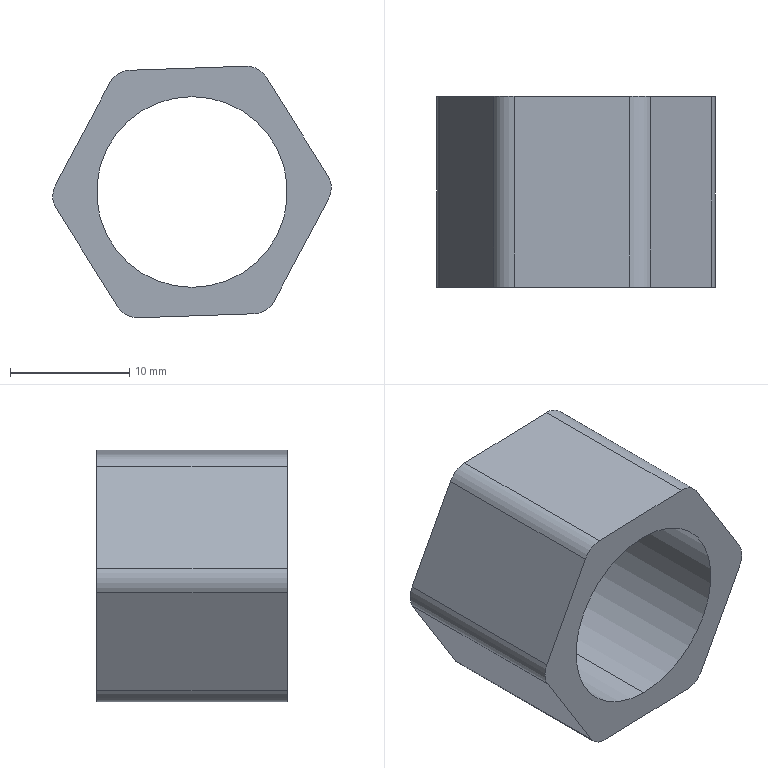Part | SolidWorks | features Fillet 2, Extrusion 1 | 1 solid | 17 faces | box 23.37 x 16 x 21.11 mm | volume 2748 mm3 | cylinder 9 | plane 8 | commonest cylinder face diameters 4 x7 16 x2
STEP:
#1=CARTESIAN_POINT('',(-4.552,16.,-10.555));
#2=VERTEX_POINT('',#1);
#3=CARTESIAN_POINT('',(-6.249,16.,-9.614));
#4=VERTEX_POINT('',#3);
#5=CARTESIAN_POINT('',(-4.552,16.,-8.555));
#6=DIRECTION('',(0.,1.,0.));
#7=DIRECTION('',(0.,0.,1.));
#8=AXIS2_PLACEMENT_3D('',#5,#6,#7);
#9=CIRCLE('',#8,2.);
#10=EDGE_CURVE('',#2,#4,#9,.T.);
#11=ORIENTED_EDGE('',*,*,#10,.F.);
#12=CARTESIAN_POINT('',(-4.552,0.,-10.555));
#13=VERTEX_POINT('',#12);
#14=CARTESIAN_POINT('',(-4.552,16.,-10.555));
#15=DIRECTION('',(0.,-1.,0.));
#16=VECTOR('',#15,1000.);
#17=LINE('',#14,#16);
#18=EDGE_CURVE('',#2,#13,#17,.T.);
#19=ORIENTED_EDGE('',*,*,#18,.T.);
#20=CARTESIAN_POINT('',(-6.249,0.,-9.614));
#21=VERTEX_POINT('',#20);
#22=CARTESIAN_POINT('',(-4.552,0.,-8.555));
#23=DIRECTION('',(0.,-1.,0.));
#24=DIRECTION('',(0.,0.,1.));
#25=AXIS2_PLACEMENT_3D('',#22,#23,#24);
#26=CIRCLE('',#25,2.);
#27=EDGE_CURVE('',#21,#13,#26,.T.);
#28=ORIENTED_EDGE('',*,*,#27,.F.);
#29=CARTESIAN_POINT('',(-6.249,16.,-9.614));
#30=DIRECTION('',(0.,-1.,0.));
#31=VECTOR('',#30,1000.);
#32=LINE('',#29,#31);
#33=EDGE_CURVE('',#4,#21,#32,.T.);
#34=ORIENTED_EDGE('',*,*,#33,.F.);
#35=EDGE_LOOP('',(#11,#19,#28,#34));
#36=FACE_OUTER_BOUND('',#35,.T.);
#37=CARTESIAN_POINT('',(-4.552,16.,-8.555));
#38=DIRECTION('',(0.,-1.,0.));
#39=DIRECTION('',(0.,0.,-1.));
#40=AXIS2_PLACEMENT_3D('',#37,#38,#39);
#41=CYLINDRICAL_SURFACE('',#40,2.);
#42=ADVANCED_FACE('',(#36),#41,.T.);
#43=CARTESIAN_POINT('',(0.,16.,-8.));
#44=VERTEX_POINT('',#43);
#45=CARTESIAN_POINT('',(0.,16.,8.));
#46=VERTEX_POINT('',#45);
#47=CARTESIAN_POINT('',(0.,16.,0.));
#48=DIRECTION('',(0.,1.,0.));
#49=DIRECTION('',(0.,0.,1.));
#50=AXIS2_PLACEMENT_3D('',#47,#48,#49);
#51=CIRCLE('',#50,8.);
#52=EDGE_CURVE('',#44,#46,#51,.T.);
#53=ORIENTED_EDGE('',*,*,#52,.T.);
#54=CARTESIAN_POINT('',(0.,0.,8.));
#55=VERTEX_POINT('',#54);
#56=CARTESIAN_POINT('',(0.,16.,8.));
#57=DIRECTION('',(0.,-1.,0.));
#58=VECTOR('',#57,1000.);
#59=LINE('',#56,#58);
#60=EDGE_CURVE('',#46,#55,#59,.T.);
#61=ORIENTED_EDGE('',*,*,#60,.T.);
#62=CARTESIAN_POINT('',(0.,0.,-8.));
#63=VERTEX_POINT('',#62);
#64=CARTESIAN_POINT('',(0.,0.,0.));
#65=DIRECTION('',(0.,1.,0.));
#66=DIRECTION('',(0.,0.,1.));
#67=AXIS2_PLACEMENT_3D('',#64,#65,#66);
#68=CIRCLE('',#67,8.);
#69=EDGE_CURVE('',#63,#55,#68,.T.);
#70=ORIENTED_EDGE('',*,*,#69,.F.);
#71=CARTESIAN_POINT('',(0.,16.,-8.));
#72=DIRECTION('',(0.,-1.,0.));
#73=VECTOR('',#72,1000.);
#74=LINE('',#71,#73);
#75=EDGE_CURVE('',#44,#63,#74,.T.);
#76=ORIENTED_EDGE('',*,*,#75,.F.);
#77=EDGE_LOOP('',(#53,#61,#70,#76));
#78=FACE_OUTER_BOUND('',#77,.T.);
#79=CARTESIAN_POINT('',(0.,16.,0.));
#80=DIRECTION('',(0.,-1.,0.));
#81=DIRECTION('',(0.,0.,-1.));
#82=AXIS2_PLACEMENT_3D('',#79,#80,#81);
#83=CYLINDRICAL_SURFACE('',#82,8.);
#84=ADVANCED_FACE('',(#78),#83,.F.);
#85=CARTESIAN_POINT('',(5.202,16.,-10.219));
#86=VERTEX_POINT('',#85);
#87=CARTESIAN_POINT('',(-4.483,16.,-10.554));
#88=VERTEX_POINT('',#87);
#89=CARTESIAN_POINT('',(6.356,16.,-10.179));
#90=DIRECTION('',(-0.9994,0.,-0.03459));
#91=VECTOR('',#90,1000.);
#92=LINE('',#89,#91);
#93=EDGE_CURVE('',#86,#88,#92,.T.);
#94=ORIENTED_EDGE('',*,*,#93,.T.);
#95=CARTESIAN_POINT('',(-4.552,16.,-8.555));
#96=DIRECTION('',(0.,1.,0.));
#97=DIRECTION('',(0.,0.,1.));
#98=AXIS2_PLACEMENT_3D('',#95,#96,#97);
#99=CIRCLE('',#98,2.);
#100=EDGE_CURVE('',#88,#2,#99,.T.);
#101=ORIENTED_EDGE('',*,*,#100,.T.);
#102=ORIENTED_EDGE('',*,*,#10,.T.);
#103=CARTESIAN_POINT('',(-11.381,16.,-1.394));
#104=VERTEX_POINT('',#103);
#105=CARTESIAN_POINT('',(-5.637,16.,-10.594));
#106=DIRECTION('',(-0.5297,0.,0.8482));
#107=VECTOR('',#106,1000.);
#108=LINE('',#105,#107);
#109=EDGE_CURVE('',#4,#104,#108,.T.);
#110=ORIENTED_EDGE('',*,*,#109,.T.);
#111=CARTESIAN_POINT('',(-11.45,16.,0.6043));
#112=VERTEX_POINT('',#111);
#113=CARTESIAN_POINT('',(-9.685,16.,-0.3352));
#114=DIRECTION('',(0.,1.,0.));
#115=DIRECTION('',(0.,0.,1.));
#116=AXIS2_PLACEMENT_3D('',#113,#114,#115);
#117=CIRCLE('',#116,2.);
#118=EDGE_CURVE('',#104,#112,#117,.T.);
#119=ORIENTED_EDGE('',*,*,#118,.T.);
#120=CARTESIAN_POINT('',(-6.898,16.,9.159));
#121=VERTEX_POINT('',#120);
#122=CARTESIAN_POINT('',(-11.993,16.,-0.415));
#123=DIRECTION('',(0.4697,0.,0.8828));
#124=VECTOR('',#123,1000.);
#125=LINE('',#122,#124);
#126=EDGE_CURVE('',#112,#121,#125,.T.);
#127=ORIENTED_EDGE('',*,*,#126,.T.);
#128=CARTESIAN_POINT('',(-5.202,16.,10.219));
#129=VERTEX_POINT('',#128);
#130=CARTESIAN_POINT('',(-5.133,16.,8.22));
#131=DIRECTION('',(0.,1.,0.));
#132=DIRECTION('',(0.,0.,1.));
#133=AXIS2_PLACEMENT_3D('',#130,#131,#132);
#134=CIRCLE('',#133,2.);
#135=EDGE_CURVE('',#121,#129,#134,.T.);
#136=ORIENTED_EDGE('',*,*,#135,.T.);
#137=CARTESIAN_POINT('',(4.483,16.,10.554));
#138=VERTEX_POINT('',#137);
#139=CARTESIAN_POINT('',(-6.356,16.,10.179));
#140=DIRECTION('',(0.9994,0.,0.03459));
#141=VECTOR('',#140,1000.);
#142=LINE('',#139,#141);
#143=EDGE_CURVE('',#129,#138,#142,.T.);
#144=ORIENTED_EDGE('',*,*,#143,.T.);
#145=CARTESIAN_POINT('',(6.249,16.,9.614));
#146=VERTEX_POINT('',#145);
#147=CARTESIAN_POINT('',(4.552,16.,8.555));
#148=DIRECTION('',(0.,1.,0.));
#149=DIRECTION('',(0.,0.,1.));
#150=AXIS2_PLACEMENT_3D('',#147,#148,#149);
#151=CIRCLE('',#150,2.);
#152=EDGE_CURVE('',#138,#146,#151,.T.);
#153=ORIENTED_EDGE('',*,*,#152,.T.);
#154=CARTESIAN_POINT('',(11.381,16.,1.394));
#155=VERTEX_POINT('',#154);
#156=CARTESIAN_POINT('',(5.637,16.,10.594));
#157=DIRECTION('',(0.5297,0.,-0.8482));
#158=VECTOR('',#157,1000.);
#159=LINE('',#156,#158);
#160=EDGE_CURVE('',#146,#155,#159,.T.);
#161=ORIENTED_EDGE('',*,*,#160,.T.);
#162=CARTESIAN_POINT('',(11.45,16.,-0.6043));
#163=VERTEX_POINT('',#162);
#164=CARTESIAN_POINT('',(9.685,16.,0.3352));
#165=DIRECTION('',(0.,1.,0.));
#166=DIRECTION('',(0.,0.,1.));
#167=AXIS2_PLACEMENT_3D('',#164,#165,#166);
#168=CIRCLE('',#167,2.);
#169=EDGE_CURVE('',#155,#163,#168,.T.);
#170=ORIENTED_EDGE('',*,*,#169,.T.);
#171=CARTESIAN_POINT('',(6.898,16.,-9.159));
#172=VERTEX_POINT('',#171);
#173=CARTESIAN_POINT('',(11.993,16.,0.415));
#174=DIRECTION('',(-0.4697,0.,-0.8828));
#175=VECTOR('',#174,1000.);
#176=LINE('',#173,#175);
#177=EDGE_CURVE('',#163,#172,#176,.T.);
#178=ORIENTED_EDGE('',*,*,#177,.T.);
#179=CARTESIAN_POINT('',(5.133,16.,-8.22));
#180=DIRECTION('',(0.,1.,0.));
#181=DIRECTION('',(0.,0.,1.));
#182=AXIS2_PLACEMENT_3D('',#179,#180,#181);
#183=CIRCLE('',#182,2.);
#184=EDGE_CURVE('',#172,#86,#183,.T.);
#185=ORIENTED_EDGE('',*,*,#184,.T.);
#186=EDGE_LOOP('',(#94,#101,#102,#110,#119,#127,#136,#144,#153,#161,#170,#178,#185));
#187=FACE_OUTER_BOUND('',#186,.T.);
#188=ORIENTED_EDGE('',*,*,#52,.F.);
#189=CARTESIAN_POINT('',(0.,16.,0.));
#190=DIRECTION('',(0.,1.,0.));
#191=DIRECTION('',(0.,0.,1.));
#192=AXIS2_PLACEMENT_3D('',#189,#190,#191);
#193=CIRCLE('',#192,8.);
#194=EDGE_CURVE('',#46,#44,#193,.T.);
#195=ORIENTED_EDGE('',*,*,#194,.F.);
#196=EDGE_LOOP('',(#188,#195));
#197=FACE_BOUND('',#196,.T.);
#198=CARTESIAN_POINT('',(0.,16.,0.));
#199=DIRECTION('',(0.,1.,0.));
#200=DIRECTION('',(0.,0.,1.));
#201=AXIS2_PLACEMENT_3D('',#198,#199,#200);
#202=PLANE('',#201);
#203=ADVANCED_FACE('',(#187,#197),#202,.T.);
#204=CARTESIAN_POINT('',(-11.381,0.,-1.394));
#205=VERTEX_POINT('',#204);
#206=CARTESIAN_POINT('',(-5.637,0.,-10.594));
#207=DIRECTION('',(-0.5297,0.,0.8482));
#208=VECTOR('',#207,1000.);
#209=LINE('',#206,#208);
#210=EDGE_CURVE('',#21,#205,#209,.T.);
#211=ORIENTED_EDGE('',*,*,#210,.F.);
#212=ORIENTED_EDGE('',*,*,#27,.T.);
#213=CARTESIAN_POINT('',(-4.483,0.,-10.554));
#214=VERTEX_POINT('',#213);
#215=CARTESIAN_POINT('',(-4.552,0.,-8.555));
#216=DIRECTION('',(0.,-1.,0.));
#217=DIRECTION('',(0.,0.,1.));
#218=AXIS2_PLACEMENT_3D('',#215,#216,#217);
#219=CIRCLE('',#218,2.);
#220=EDGE_CURVE('',#13,#214,#219,.T.);
#221=ORIENTED_EDGE('',*,*,#220,.T.);
#222=CARTESIAN_POINT('',(5.202,0.,-10.219));
#223=VERTEX_POINT('',#222);
#224=CARTESIAN_POINT('',(6.356,0.,-10.179));
#225=DIRECTION('',(-0.9994,0.,-0.03459));
#226=VECTOR('',#225,1000.);
#227=LINE('',#224,#226);
#228=EDGE_CURVE('',#223,#214,#227,.T.);
#229=ORIENTED_EDGE('',*,*,#228,.F.);
#230=CARTESIAN_POINT('',(6.898,0.,-9.159));
#231=VERTEX_POINT('',#230);
#232=CARTESIAN_POINT('',(5.133,0.,-8.22));
#233=DIRECTION('',(0.,-1.,0.));
#234=DIRECTION('',(0.,0.,1.));
#235=AXIS2_PLACEMENT_3D('',#232,#233,#234);
#236=CIRCLE('',#235,2.);
#237=EDGE_CURVE('',#223,#231,#236,.T.);
#238=ORIENTED_EDGE('',*,*,#237,.T.);
#239=CARTESIAN_POINT('',(11.45,0.,-0.6043));
#240=VERTEX_POINT('',#239);
#241=CARTESIAN_POINT('',(11.993,0.,0.415));
#242=DIRECTION('',(-0.4697,0.,-0.8828));
#243=VECTOR('',#242,1000.);
#244=LINE('',#241,#243);
#245=EDGE_CURVE('',#240,#231,#244,.T.);
#246=ORIENTED_EDGE('',*,*,#245,.F.);
#247=CARTESIAN_POINT('',(11.381,0.,1.394));
#248=VERTEX_POINT('',#247);
#249=CARTESIAN_POINT('',(9.685,0.,0.3352));
#250=DIRECTION('',(0.,-1.,0.));
#251=DIRECTION('',(0.,0.,1.));
#252=AXIS2_PLACEMENT_3D('',#249,#250,#251);
#253=CIRCLE('',#252,2.);
#254=EDGE_CURVE('',#240,#248,#253,.T.);
#255=ORIENTED_EDGE('',*,*,#254,.T.);
#256=CARTESIAN_POINT('',(6.249,0.,9.614));
#257=VERTEX_POINT('',#256);
#258=CARTESIAN_POINT('',(5.637,0.,10.594));
#259=DIRECTION('',(0.5297,0.,-0.8482));
#260=VECTOR('',#259,1000.);
#261=LINE('',#258,#260);
#262=EDGE_CURVE('',#257,#248,#261,.T.);
#263=ORIENTED_EDGE('',*,*,#262,.F.);
#264=CARTESIAN_POINT('',(4.483,0.,10.554));
#265=VERTEX_POINT('',#264);
#266=CARTESIAN_POINT('',(4.552,0.,8.555));
#267=DIRECTION('',(0.,-1.,0.));
#268=DIRECTION('',(0.,0.,1.));
#269=AXIS2_PLACEMENT_3D('',#266,#267,#268);
#270=CIRCLE('',#269,2.);
#271=EDGE_CURVE('',#257,#265,#270,.T.);
#272=ORIENTED_EDGE('',*,*,#271,.T.);
#273=CARTESIAN_POINT('',(-5.202,0.,10.219));
#274=VERTEX_POINT('',#273);
#275=CARTESIAN_POINT('',(-6.356,0.,10.179));
#276=DIRECTION('',(0.9994,0.,0.03459));
#277=VECTOR('',#276,1000.);
#278=LINE('',#275,#277);
#279=EDGE_CURVE('',#274,#265,#278,.T.);
#280=ORIENTED_EDGE('',*,*,#279,.F.);
#281=CARTESIAN_POINT('',(-6.898,0.,9.159));
#282=VERTEX_POINT('',#281);
#283=CARTESIAN_POINT('',(-5.133,0.,8.22));
#284=DIRECTION('',(0.,-1.,0.));
#285=DIRECTION('',(0.,0.,1.));
#286=AXIS2_PLACEMENT_3D('',#283,#284,#285);
#287=CIRCLE('',#286,2.);
#288=EDGE_CURVE('',#274,#282,#287,.T.);
#289=ORIENTED_EDGE('',*,*,#288,.T.);
#290=CARTESIAN_POINT('',(-11.45,0.,0.6043));
#291=VERTEX_POINT('',#290);
#292=CARTESIAN_POINT('',(-11.993,0.,-0.415));
#293=DIRECTION('',(0.4697,0.,0.8828));
#294=VECTOR('',#293,1000.);
#295=LINE('',#292,#294);
#296=EDGE_CURVE('',#291,#282,#295,.T.);
#297=ORIENTED_EDGE('',*,*,#296,.F.);
#298=CARTESIAN_POINT('',(-9.685,0.,-0.3352));
#299=DIRECTION('',(0.,-1.,0.));
#300=DIRECTION('',(0.,0.,1.));
#301=AXIS2_PLACEMENT_3D('',#298,#299,#300);
#302=CIRCLE('',#301,2.);
#303=EDGE_CURVE('',#291,#205,#302,.T.);
#304=ORIENTED_EDGE('',*,*,#303,.T.);
#305=EDGE_LOOP('',(#211,#212,#221,#229,#238,#246,#255,#263,#272,#280,#289,#297,#304));
#306=FACE_OUTER_BOUND('',#305,.T.);
#307=ORIENTED_EDGE('',*,*,#69,.T.);
#308=CARTESIAN_POINT('',(0.,0.,0.));
#309=DIRECTION('',(0.,1.,0.));
#310=DIRECTION('',(0.,0.,1.));
#311=AXIS2_PLACEMENT_3D('',#308,#309,#310);
#312=CIRCLE('',#311,8.);
#313=EDGE_CURVE('',#55,#63,#312,.T.);
#314=ORIENTED_EDGE('',*,*,#313,.T.);
#315=EDGE_LOOP('',(#307,#314));
#316=FACE_BOUND('',#315,.T.);
#317=CARTESIAN_POINT('',(0.,0.,0.));
#318=DIRECTION('',(0.,1.,0.));
#319=DIRECTION('',(0.,0.,1.));
#320=AXIS2_PLACEMENT_3D('',#317,#318,#319);
#321=PLANE('',#320);
#322=ADVANCED_FACE('',(#306,#316),#321,.F.);
#323=ORIENTED_EDGE('',*,*,#143,.F.);
#324=CARTESIAN_POINT('',(-5.202,16.,10.219));
#325=DIRECTION('',(0.,-1.,0.));
#326=VECTOR('',#325,1000.);
#327=LINE('',#324,#326);
#328=EDGE_CURVE('',#129,#274,#327,.T.);
#329=ORIENTED_EDGE('',*,*,#328,.T.);
#330=ORIENTED_EDGE('',*,*,#279,.T.);
#331=CARTESIAN_POINT('',(4.483,16.,10.554));
#332=DIRECTION('',(0.,1.,0.));
#333=VECTOR('',#332,1000.);
#334=LINE('',#331,#333);
#335=EDGE_CURVE('',#265,#138,#334,.T.);
#336=ORIENTED_EDGE('',*,*,#335,.T.);
#337=EDGE_LOOP('',(#323,#329,#330,#336));
#338=FACE_OUTER_BOUND('',#337,.T.);
#339=CARTESIAN_POINT('',(-6.356,16.,10.179));
#340=DIRECTION('',(0.03459,0.,-0.9994));
#341=DIRECTION('',(-0.9994,0.,-0.03459));
#342=AXIS2_PLACEMENT_3D('',#339,#340,#341);
#343=PLANE('',#342);
#344=ADVANCED_FACE('',(#338),#343,.F.);
#345=ORIENTED_EDGE('',*,*,#262,.T.);
#346=CARTESIAN_POINT('',(11.381,16.,1.394));
#347=DIRECTION('',(0.,1.,0.));
#348=VECTOR('',#347,1000.);
#349=LINE('',#346,#348);
#350=EDGE_CURVE('',#248,#155,#349,.T.);
#351=ORIENTED_EDGE('',*,*,#350,.T.);
#352=ORIENTED_EDGE('',*,*,#160,.F.);
#353=CARTESIAN_POINT('',(6.249,16.,9.614));
#354=DIRECTION('',(0.,-1.,0.));
#355=VECTOR('',#354,1000.);
#356=LINE('',#353,#355);
#357=EDGE_CURVE('',#146,#257,#356,.T.);
#358=ORIENTED_EDGE('',*,*,#357,.T.);
#359=EDGE_LOOP('',(#345,#351,#352,#358));
#360=FACE_OUTER_BOUND('',#359,.T.);
#361=CARTESIAN_POINT('',(5.637,16.,10.594));
#362=DIRECTION('',(-0.8482,0.,-0.5297));
#363=DIRECTION('',(-0.5297,0.,0.8482));
#364=AXIS2_PLACEMENT_3D('',#361,#362,#363);
#365=PLANE('',#364);
#366=ADVANCED_FACE('',(#360),#365,.F.);
#367=ORIENTED_EDGE('',*,*,#245,.T.);
#368=CARTESIAN_POINT('',(6.898,16.,-9.159));
#369=DIRECTION('',(0.,1.,0.));
#370=VECTOR('',#369,1000.);
#371=LINE('',#368,#370);
#372=EDGE_CURVE('',#231,#172,#371,.T.);
#373=ORIENTED_EDGE('',*,*,#372,.T.);
#374=ORIENTED_EDGE('',*,*,#177,.F.);
#375=CARTESIAN_POINT('',(11.45,16.,-0.6043));
#376=DIRECTION('',(0.,-1.,0.));
#377=VECTOR('',#376,1000.);
#378=LINE('',#375,#377);
#379=EDGE_CURVE('',#163,#240,#378,.T.);
#380=ORIENTED_EDGE('',*,*,#379,.T.);
#381=EDGE_LOOP('',(#367,#373,#374,#380));
#382=FACE_OUTER_BOUND('',#381,.T.);
#383=CARTESIAN_POINT('',(11.993,16.,0.415));
#384=DIRECTION('',(-0.8828,0.,0.4697));
#385=DIRECTION('',(0.4697,0.,0.8828));
#386=AXIS2_PLACEMENT_3D('',#383,#384,#385);
#387=PLANE('',#386);
#388=ADVANCED_FACE('',(#382),#387,.F.);
#389=ORIENTED_EDGE('',*,*,#228,.T.);
#390=CARTESIAN_POINT('',(-4.483,16.,-10.554));
#391=DIRECTION('',(0.,1.,0.));
#392=VECTOR('',#391,1000.);
#393=LINE('',#390,#392);
#394=EDGE_CURVE('',#214,#88,#393,.T.);
#395=ORIENTED_EDGE('',*,*,#394,.T.);
#396=ORIENTED_EDGE('',*,*,#93,.F.);
#397=CARTESIAN_POINT('',(5.202,16.,-10.219));
#398=DIRECTION('',(0.,-1.,0.));
#399=VECTOR('',#398,1000.);
#400=LINE('',#397,#399);
#401=EDGE_CURVE('',#86,#223,#400,.T.);
#402=ORIENTED_EDGE('',*,*,#401,.T.);
#403=EDGE_LOOP('',(#389,#395,#396,#402));
#404=FACE_OUTER_BOUND('',#403,.T.);
#405=CARTESIAN_POINT('',(6.356,16.,-10.179));
#406=DIRECTION('',(-0.03459,0.,0.9994));
#407=DIRECTION('',(0.9994,0.,0.03459));
#408=AXIS2_PLACEMENT_3D('',#405,#406,#407);
#409=PLANE('',#408);
#410=ADVANCED_FACE('',(#404),#409,.F.);
#411=ORIENTED_EDGE('',*,*,#109,.F.);
#412=ORIENTED_EDGE('',*,*,#33,.T.);
#413=ORIENTED_EDGE('',*,*,#210,.T.);
#414=CARTESIAN_POINT('',(-11.381,16.,-1.394));
#415=DIRECTION('',(0.,1.,0.));
#416=VECTOR('',#415,1000.);
#417=LINE('',#414,#416);
#418=EDGE_CURVE('',#205,#104,#417,.T.);
#419=ORIENTED_EDGE('',*,*,#418,.T.);
#420=EDGE_LOOP('',(#411,#412,#413,#419));
#421=FACE_OUTER_BOUND('',#420,.T.);
#422=CARTESIAN_POINT('',(-5.637,16.,-10.594));
#423=DIRECTION('',(0.8482,0.,0.5297));
#424=DIRECTION('',(0.5297,0.,-0.8482));
#425=AXIS2_PLACEMENT_3D('',#422,#423,#424);
#426=PLANE('',#425);
#427=ADVANCED_FACE('',(#421),#426,.F.);
#428=ORIENTED_EDGE('',*,*,#126,.F.);
#429=CARTESIAN_POINT('',(-11.45,16.,0.6043));
#430=DIRECTION('',(0.,-1.,0.));
#431=VECTOR('',#430,1000.);
#432=LINE('',#429,#431);
#433=EDGE_CURVE('',#112,#291,#432,.T.);
#434=ORIENTED_EDGE('',*,*,#433,.T.);
#435=ORIENTED_EDGE('',*,*,#296,.T.);
#436=CARTESIAN_POINT('',(-6.898,16.,9.159));
#437=DIRECTION('',(0.,1.,0.));
#438=VECTOR('',#437,1000.);
#439=LINE('',#436,#438);
#440=EDGE_CURVE('',#282,#121,#439,.T.);
#441=ORIENTED_EDGE('',*,*,#440,.T.);
#442=EDGE_LOOP('',(#428,#434,#435,#441));
#443=FACE_OUTER_BOUND('',#442,.T.);
#444=CARTESIAN_POINT('',(-11.993,16.,-0.415));
#445=DIRECTION('',(0.8828,0.,-0.4697));
#446=DIRECTION('',(-0.4697,0.,-0.8828));
#447=AXIS2_PLACEMENT_3D('',#444,#445,#446);
#448=PLANE('',#447);
#449=ADVANCED_FACE('',(#443),#448,.F.);
#450=ORIENTED_EDGE('',*,*,#60,.F.);
#451=ORIENTED_EDGE('',*,*,#194,.T.);
#452=ORIENTED_EDGE('',*,*,#75,.T.);
#453=ORIENTED_EDGE('',*,*,#313,.F.);
#454=EDGE_LOOP('',(#450,#451,#452,#453));
#455=FACE_OUTER_BOUND('',#454,.T.);
#456=CARTESIAN_POINT('',(0.,16.,0.));
#457=DIRECTION('',(0.,-1.,0.));
#458=DIRECTION('',(0.,0.,-1.));
#459=AXIS2_PLACEMENT_3D('',#456,#457,#458);
#460=CYLINDRICAL_SURFACE('',#459,8.);
#461=ADVANCED_FACE('',(#455),#460,.F.);
#462=ORIENTED_EDGE('',*,*,#152,.F.);
#463=ORIENTED_EDGE('',*,*,#335,.F.);
#464=ORIENTED_EDGE('',*,*,#271,.F.);
#465=ORIENTED_EDGE('',*,*,#357,.F.);
#466=EDGE_LOOP('',(#462,#463,#464,#465));
#467=FACE_OUTER_BOUND('',#466,.T.);
#468=CARTESIAN_POINT('',(4.552,16.,8.555));
#469=DIRECTION('',(0.,-1.,0.));
#470=DIRECTION('',(0.,0.,-1.));
#471=AXIS2_PLACEMENT_3D('',#468,#469,#470);
#472=CYLINDRICAL_SURFACE('',#471,2.);
#473=ADVANCED_FACE('',(#467),#472,.T.);
#474=ORIENTED_EDGE('',*,*,#18,.F.);
#475=ORIENTED_EDGE('',*,*,#100,.F.);
#476=ORIENTED_EDGE('',*,*,#394,.F.);
#477=ORIENTED_EDGE('',*,*,#220,.F.);
#478=EDGE_LOOP('',(#474,#475,#476,#477));
#479=FACE_OUTER_BOUND('',#478,.T.);
#480=CARTESIAN_POINT('',(-4.552,16.,-8.555));
#481=DIRECTION('',(0.,-1.,0.));
#482=DIRECTION('',(0.,0.,-1.));
#483=AXIS2_PLACEMENT_3D('',#480,#481,#482);
#484=CYLINDRICAL_SURFACE('',#483,2.);
#485=ADVANCED_FACE('',(#479),#484,.T.);
#486=ORIENTED_EDGE('',*,*,#118,.F.);
#487=ORIENTED_EDGE('',*,*,#418,.F.);
#488=ORIENTED_EDGE('',*,*,#303,.F.);
#489=ORIENTED_EDGE('',*,*,#433,.F.);
#490=EDGE_LOOP('',(#486,#487,#488,#489));
#491=FACE_OUTER_BOUND('',#490,.T.);
#492=CARTESIAN_POINT('',(-9.685,16.,-0.3352));
#493=DIRECTION('',(0.,-1.,0.));
#494=DIRECTION('',(0.,0.,-1.));
#495=AXIS2_PLACEMENT_3D('',#492,#493,#494);
#496=CYLINDRICAL_SURFACE('',#495,2.);
#497=ADVANCED_FACE('',(#491),#496,.T.);
#498=ORIENTED_EDGE('',*,*,#135,.F.);
#499=ORIENTED_EDGE('',*,*,#440,.F.);
#500=ORIENTED_EDGE('',*,*,#288,.F.);
#501=ORIENTED_EDGE('',*,*,#328,.F.);
#502=EDGE_LOOP('',(#498,#499,#500,#501));
#503=FACE_OUTER_BOUND('',#502,.T.);
#504=CARTESIAN_POINT('',(-5.133,16.,8.22));
#505=DIRECTION('',(0.,-1.,0.));
#506=DIRECTION('',(0.,0.,-1.));
#507=AXIS2_PLACEMENT_3D('',#504,#505,#506);
#508=CYLINDRICAL_SURFACE('',#507,2.);
#509=ADVANCED_FACE('',(#503),#508,.T.);
#510=ORIENTED_EDGE('',*,*,#184,.F.);
#511=ORIENTED_EDGE('',*,*,#372,.F.);
#512=ORIENTED_EDGE('',*,*,#237,.F.);
#513=ORIENTED_EDGE('',*,*,#401,.F.);
#514=EDGE_LOOP('',(#510,#511,#512,#513));
#515=FACE_OUTER_BOUND('',#514,.T.);
#516=CARTESIAN_POINT('',(5.133,16.,-8.22));
#517=DIRECTION('',(0.,-1.,0.));
#518=DIRECTION('',(0.,0.,-1.));
#519=AXIS2_PLACEMENT_3D('',#516,#517,#518);
#520=CYLINDRICAL_SURFACE('',#519,2.);
#521=ADVANCED_FACE('',(#515),#520,.T.);
#522=ORIENTED_EDGE('',*,*,#169,.F.);
#523=ORIENTED_EDGE('',*,*,#350,.F.);
#524=ORIENTED_EDGE('',*,*,#254,.F.);
#525=ORIENTED_EDGE('',*,*,#379,.F.);
#526=EDGE_LOOP('',(#522,#523,#524,#525));
#527=FACE_OUTER_BOUND('',#526,.T.);
#528=CARTESIAN_POINT('',(9.685,16.,0.3352));
#529=DIRECTION('',(0.,-1.,0.));
#530=DIRECTION('',(0.,0.,-1.));
#531=AXIS2_PLACEMENT_3D('',#528,#529,#530);
#532=CYLINDRICAL_SURFACE('',#531,2.);
#533=ADVANCED_FACE('',(#527),#532,.T.);
#534=CLOSED_SHELL('',(#42,#84,#203,#322,#344,#366,#388,#410,#427,#449,#461,#473,#485,#497,#509,#521,#533));
#535=MANIFOLD_SOLID_BREP('',#534);
#536=CARTESIAN_POINT('',(0.,0.,0.));
#537=DIRECTION('',(0.,0.,1.));
#538=DIRECTION('',(1.,0.,0.));
#539=AXIS2_PLACEMENT_3D('',#536,#537,#538);
#540=(LENGTH_UNIT()NAMED_UNIT(*)SI_UNIT(.MILLI.,.METRE.));
#541=UNCERTAINTY_MEASURE_WITH_UNIT(LENGTH_MEASURE(0.00001),#540,'','');
#542=(NAMED_UNIT(*)PLANE_ANGLE_UNIT()SI_UNIT($,.RADIAN.));
#543=(NAMED_UNIT(*)SI_UNIT($,.STERADIAN.)SOLID_ANGLE_UNIT());
#544=(GEOMETRIC_REPRESENTATION_CONTEXT(3)GLOBAL_UNCERTAINTY_ASSIGNED_CONTEXT((#541))GLOBAL_UNIT_ASSIGNED_CONTEXT((#540,#542,#543))REPRESENTATION_CONTEXT('',''));
#545=ADVANCED_BREP_SHAPE_REPRESENTATION('',(#535,#539),#544);